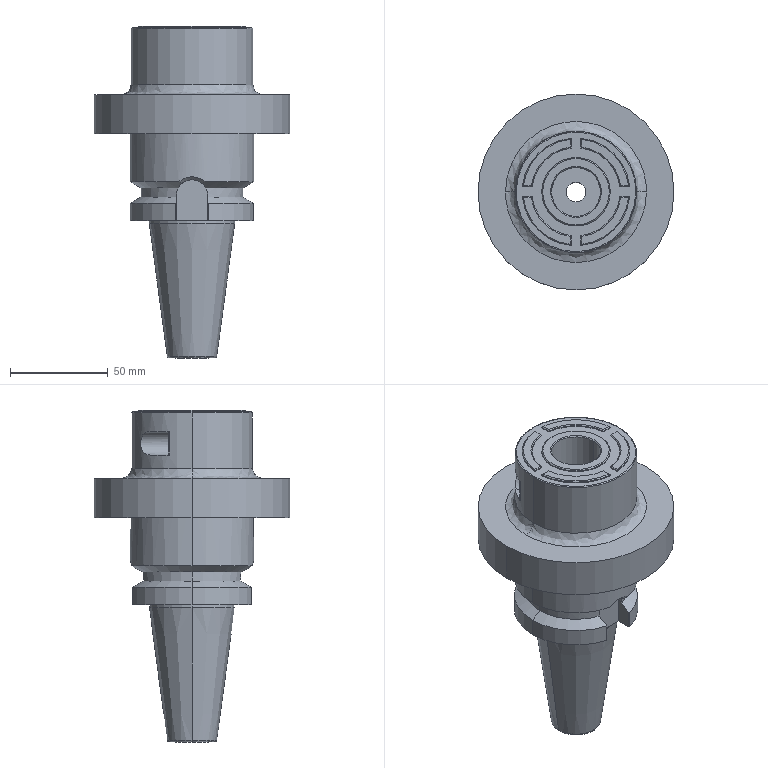Part | SolidWorks | features BaseBody 1 | 1 solid | 122 faces | box 100 x 100 x 169.5 mm | volume 348963 mm3 | plane 47 | cylinder 45 | cone 22 | spline 8 | commonest cylinder face diameters 16 x6 63 x5 45 x4 55 x4 52 x3 8 x2